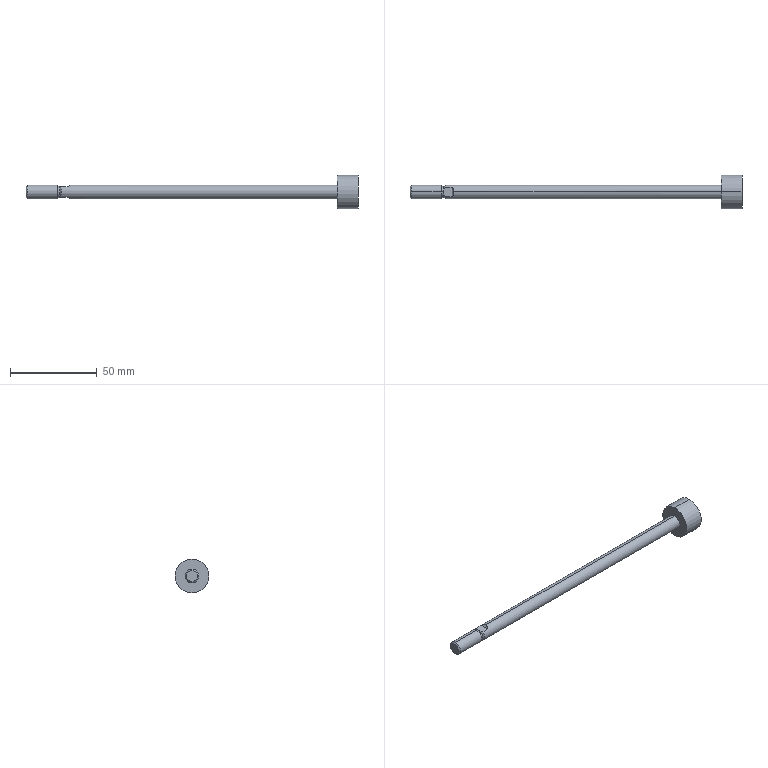Part | SolidWorks | features BaseBody 1 | 1 solid | 22 faces | box 191.2 x 19.5 x 19.5 mm | volume 12515 mm3 | plane 10 | cylinder 8 | cone 4 | commonest cylinder face diameters 8 x4 6.4 x2 19.5 x2
STEP:
#1=CARTESIAN_POINT('',(-24.5,-1.114,3.));
#2=VERTEX_POINT('',#1);
#3=CARTESIAN_POINT('',(-23.7,-2.646,3.));
#4=VERTEX_POINT('',#3);
#5=CARTESIAN_POINT('',(-24.5,-1.114,3.));
#6=CARTESIAN_POINT('',(-24.457,-1.239,3.));
#7=CARTESIAN_POINT('',(-24.38,-1.431,3.));
#8=CARTESIAN_POINT('',(-24.27,-1.665,3.));
#9=CARTESIAN_POINT('',(-24.21,-1.784,3.));
#10=CARTESIAN_POINT('',(-24.179,-1.844,3.));
#11=CARTESIAN_POINT('',(-24.165,-1.87,3.));
#12=CARTESIAN_POINT('',(-24.156,-1.887,3.));
#13=CARTESIAN_POINT('',(-24.151,-1.897,3.));
#14=CARTESIAN_POINT('',(-24.022,-2.137,3.));
#15=CARTESIAN_POINT('',(-23.873,-2.384,3.));
#16=CARTESIAN_POINT('',(-23.7,-2.646,3.));
#17=B_SPLINE_CURVE_WITH_KNOTS('',3,(#5,#6,#7,#8,#9,#10,#11,#12,#13,#14,#15,#16),.UNSPECIFIED.,.F.,.F.,(4,1,1,1,1,2,2,4),(0.,0.25,0.375,0.4375,0.4688,0.4844,0.5,1.),.UNSPECIFIED.);
#18=EDGE_CURVE('',#2,#4,#17,.T.);
#19=ORIENTED_EDGE('',*,*,#18,.T.);
#20=CARTESIAN_POINT('',(-19.7,-2.646,3.));
#21=VERTEX_POINT('',#20);
#22=CARTESIAN_POINT('',(-23.7,-2.646,3.));
#23=DIRECTION('',(1.,0.,0.));
#24=VECTOR('',#23,1000.);
#25=LINE('',#22,#24);
#26=EDGE_CURVE('',#4,#21,#25,.T.);
#27=ORIENTED_EDGE('',*,*,#26,.T.);
#28=CARTESIAN_POINT('',(-19.7,2.646,3.));
#29=VERTEX_POINT('',#28);
#30=CARTESIAN_POINT('',(-19.7,2.646,3.));
#31=DIRECTION('',(0.,-1.,0.));
#32=VECTOR('',#31,1000.);
#33=LINE('',#30,#32);
#34=EDGE_CURVE('',#29,#21,#33,.T.);
#35=ORIENTED_EDGE('',*,*,#34,.F.);
#36=CARTESIAN_POINT('',(-23.7,2.646,3.));
#37=VERTEX_POINT('',#36);
#38=CARTESIAN_POINT('',(-19.7,2.646,3.));
#39=DIRECTION('',(-1.,0.,0.));
#40=VECTOR('',#39,1000.);
#41=LINE('',#38,#40);
#42=EDGE_CURVE('',#29,#37,#41,.T.);
#43=ORIENTED_EDGE('',*,*,#42,.T.);
#44=CARTESIAN_POINT('',(-24.5,1.114,3.));
#45=VERTEX_POINT('',#44);
#46=CARTESIAN_POINT('',(-23.7,2.646,3.));
#47=CARTESIAN_POINT('',(-23.787,2.515,3.));
#48=CARTESIAN_POINT('',(-23.907,2.324,3.));
#49=CARTESIAN_POINT('',(-24.033,2.11,3.));
#50=CARTESIAN_POINT('',(-24.091,2.006,3.));
#51=CARTESIAN_POINT('',(-24.119,1.955,3.));
#52=CARTESIAN_POINT('',(-24.131,1.933,3.));
#53=CARTESIAN_POINT('',(-24.139,1.918,3.));
#54=CARTESIAN_POINT('',(-24.142,1.912,3.));
#55=CARTESIAN_POINT('',(-24.295,1.627,3.));
#56=CARTESIAN_POINT('',(-24.413,1.363,3.));
#57=CARTESIAN_POINT('',(-24.5,1.114,3.));
#58=B_SPLINE_CURVE_WITH_KNOTS('',3,(#46,#47,#48,#49,#50,#51,#52,#53,#54,#55,#56,#57),.UNSPECIFIED.,.F.,.F.,(4,1,1,1,1,2,2,4),(0.,0.25,0.375,0.4375,0.4688,0.4844,0.5,1.),.UNSPECIFIED.);
#59=EDGE_CURVE('',#37,#45,#58,.T.);
#60=ORIENTED_EDGE('',*,*,#59,.T.);
#61=CARTESIAN_POINT('',(-24.5,1.114,3.));
#62=DIRECTION('',(0.,-1.,0.));
#63=VECTOR('',#62,1000.);
#64=LINE('',#61,#63);
#65=EDGE_CURVE('',#45,#2,#64,.T.);
#66=ORIENTED_EDGE('',*,*,#65,.T.);
#67=EDGE_LOOP('',(#19,#27,#35,#43,#60,#66));
#68=FACE_OUTER_BOUND('',#67,.T.);
#69=CARTESIAN_POINT('',(-19.7,8.,3.));
#70=DIRECTION('',(0.,0.,1.));
#71=DIRECTION('',(1.,0.,0.));
#72=AXIS2_PLACEMENT_3D('',#69,#70,#71);
#73=PLANE('',#72);
#74=ADVANCED_FACE('',(#68),#73,.T.);
#75=CARTESIAN_POINT('',(-18.7,0.,4.));
#76=VERTEX_POINT('',#75);
#77=CARTESIAN_POINT('',(-19.7,-2.646,3.));
#78=CARTESIAN_POINT('',(-19.378,-2.281,3.322));
#79=CARTESIAN_POINT('',(-19.131,-1.87,3.569));
#80=CARTESIAN_POINT('',(-18.786,-0.9587,3.914));
#81=CARTESIAN_POINT('',(-18.7,-0.4873,4.));
#82=CARTESIAN_POINT('',(-18.7,0.,4.));
#83=B_SPLINE_CURVE_WITH_KNOTS('',3,(#77,#78,#79,#80,#81,#82),.UNSPECIFIED.,.F.,.F.,(4,2,4),(0.,0.5,1.),.UNSPECIFIED.);
#84=EDGE_CURVE('',#21,#76,#83,.T.);
#85=ORIENTED_EDGE('',*,*,#84,.T.);
#86=CARTESIAN_POINT('',(-18.7,0.,4.));
#87=CARTESIAN_POINT('',(-18.7,0.487,4.));
#88=CARTESIAN_POINT('',(-18.786,0.9587,3.914));
#89=CARTESIAN_POINT('',(-19.13,1.87,3.57));
#90=CARTESIAN_POINT('',(-19.378,2.28,3.322));
#91=CARTESIAN_POINT('',(-19.7,2.646,3.));
#92=B_SPLINE_CURVE_WITH_KNOTS('',3,(#86,#87,#88,#89,#90,#91),.UNSPECIFIED.,.F.,.F.,(4,2,4),(0.,0.5,1.),.UNSPECIFIED.);
#93=EDGE_CURVE('',#76,#29,#92,.T.);
#94=ORIENTED_EDGE('',*,*,#93,.T.);
#95=ORIENTED_EDGE('',*,*,#34,.T.);
#96=EDGE_LOOP('',(#85,#94,#95));
#97=FACE_OUTER_BOUND('',#96,.T.);
#98=CARTESIAN_POINT('',(-13.7,8.,9.));
#99=DIRECTION('',(-0.7071,0.,0.7071));
#100=DIRECTION('',(0.,1.,0.));
#101=AXIS2_PLACEMENT_3D('',#98,#99,#100);
#102=PLANE('',#101);
#103=ADVANCED_FACE('',(#97),#102,.T.);
#104=CARTESIAN_POINT('',(-24.5,0.,3.2));
#105=VERTEX_POINT('',#104);
#106=CARTESIAN_POINT('',(-24.5,0.,0.));
#107=DIRECTION('',(1.,0.,0.));
#108=DIRECTION('',(0.,0.348,0.9375));
#109=AXIS2_PLACEMENT_3D('',#106,#107,#108);
#110=CIRCLE('',#109,3.2);
#111=EDGE_CURVE('',#45,#105,#110,.T.);
#112=ORIENTED_EDGE('',*,*,#111,.T.);
#113=CARTESIAN_POINT('',(-24.5,0.,0.));
#114=DIRECTION('',(1.,0.,0.));
#115=DIRECTION('',(0.,0.348,0.9375));
#116=AXIS2_PLACEMENT_3D('',#113,#114,#115);
#117=CIRCLE('',#116,3.2);
#118=EDGE_CURVE('',#105,#2,#117,.T.);
#119=ORIENTED_EDGE('',*,*,#118,.T.);
#120=ORIENTED_EDGE('',*,*,#65,.F.);
#121=EDGE_LOOP('',(#112,#119,#120));
#122=FACE_OUTER_BOUND('',#121,.T.);
#123=CARTESIAN_POINT('',(-24.5,8.,3.));
#124=DIRECTION('',(1.,0.,0.));
#125=DIRECTION('',(0.,1.,0.));
#126=AXIS2_PLACEMENT_3D('',#123,#124,#125);
#127=PLANE('',#126);
#128=ADVANCED_FACE('',(#122),#127,.T.);
#129=CARTESIAN_POINT('',(-24.5,-1.114,-3.));
#130=VERTEX_POINT('',#129);
#131=CARTESIAN_POINT('',(-24.5,0.,-3.2));
#132=VERTEX_POINT('',#131);
#133=CARTESIAN_POINT('',(-24.5,0.,0.));
#134=DIRECTION('',(1.,0.,0.));
#135=DIRECTION('',(0.,-0.348,-0.9375));
#136=AXIS2_PLACEMENT_3D('',#133,#134,#135);
#137=CIRCLE('',#136,3.2);
#138=EDGE_CURVE('',#130,#132,#137,.T.);
#139=ORIENTED_EDGE('',*,*,#138,.T.);
#140=CARTESIAN_POINT('',(-24.5,1.114,-3.));
#141=VERTEX_POINT('',#140);
#142=CARTESIAN_POINT('',(-24.5,0.,0.));
#143=DIRECTION('',(1.,0.,0.));
#144=DIRECTION('',(0.,-0.348,-0.9375));
#145=AXIS2_PLACEMENT_3D('',#142,#143,#144);
#146=CIRCLE('',#145,3.2);
#147=EDGE_CURVE('',#132,#141,#146,.T.);
#148=ORIENTED_EDGE('',*,*,#147,.T.);
#149=CARTESIAN_POINT('',(-24.5,1.114,-3.));
#150=DIRECTION('',(0.,-1.,0.));
#151=VECTOR('',#150,1000.);
#152=LINE('',#149,#151);
#153=EDGE_CURVE('',#141,#130,#152,.T.);
#154=ORIENTED_EDGE('',*,*,#153,.T.);
#155=EDGE_LOOP('',(#139,#148,#154));
#156=FACE_OUTER_BOUND('',#155,.T.);
#157=CARTESIAN_POINT('',(-24.5,8.,-4.8));
#158=DIRECTION('',(1.,0.,0.));
#159=DIRECTION('',(0.,1.,0.));
#160=AXIS2_PLACEMENT_3D('',#157,#158,#159);
#161=PLANE('',#160);
#162=ADVANCED_FACE('',(#156),#161,.T.);
#163=CARTESIAN_POINT('',(-23.7,2.646,-3.));
#164=VERTEX_POINT('',#163);
#165=CARTESIAN_POINT('',(-24.5,1.114,-3.));
#166=CARTESIAN_POINT('',(-24.457,1.239,-3.));
#167=CARTESIAN_POINT('',(-24.38,1.431,-3.));
#168=CARTESIAN_POINT('',(-24.27,1.665,-3.));
#169=CARTESIAN_POINT('',(-24.21,1.784,-3.));
#170=CARTESIAN_POINT('',(-24.179,1.844,-3.));
#171=CARTESIAN_POINT('',(-24.165,1.87,-3.));
#172=CARTESIAN_POINT('',(-24.156,1.887,-3.));
#173=CARTESIAN_POINT('',(-24.151,1.897,-3.));
#174=CARTESIAN_POINT('',(-24.022,2.137,-3.));
#175=CARTESIAN_POINT('',(-23.873,2.384,-3.));
#176=CARTESIAN_POINT('',(-23.7,2.646,-3.));
#177=B_SPLINE_CURVE_WITH_KNOTS('',3,(#165,#166,#167,#168,#169,#170,#171,#172,#173,#174,#175,#176),.UNSPECIFIED.,.F.,.F.,(4,1,1,1,1,2,2,4),(0.,0.25,0.375,0.4375,0.4687,0.4844,0.5,1.),.UNSPECIFIED.);
#178=EDGE_CURVE('',#141,#164,#177,.T.);
#179=ORIENTED_EDGE('',*,*,#178,.T.);
#180=CARTESIAN_POINT('',(-19.7,2.646,-3.));
#181=VERTEX_POINT('',#180);
#182=CARTESIAN_POINT('',(-23.7,2.646,-3.));
#183=DIRECTION('',(1.,0.,0.));
#184=VECTOR('',#183,1000.);
#185=LINE('',#182,#184);
#186=EDGE_CURVE('',#164,#181,#185,.T.);
#187=ORIENTED_EDGE('',*,*,#186,.T.);
#188=CARTESIAN_POINT('',(-19.7,-2.646,-3.));
#189=VERTEX_POINT('',#188);
#190=CARTESIAN_POINT('',(-19.7,2.646,-3.));
#191=DIRECTION('',(0.,-1.,0.));
#192=VECTOR('',#191,1000.);
#193=LINE('',#190,#192);
#194=EDGE_CURVE('',#181,#189,#193,.T.);
#195=ORIENTED_EDGE('',*,*,#194,.T.);
#196=CARTESIAN_POINT('',(-23.7,-2.646,-3.));
#197=VERTEX_POINT('',#196);
#198=CARTESIAN_POINT('',(-19.7,-2.646,-3.));
#199=DIRECTION('',(-1.,0.,0.));
#200=VECTOR('',#199,1000.);
#201=LINE('',#198,#200);
#202=EDGE_CURVE('',#189,#197,#201,.T.);
#203=ORIENTED_EDGE('',*,*,#202,.T.);
#204=CARTESIAN_POINT('',(-23.7,-2.646,-3.));
#205=CARTESIAN_POINT('',(-23.787,-2.515,-3.));
#206=CARTESIAN_POINT('',(-23.907,-2.324,-3.));
#207=CARTESIAN_POINT('',(-24.033,-2.11,-3.));
#208=CARTESIAN_POINT('',(-24.091,-2.006,-3.));
#209=CARTESIAN_POINT('',(-24.119,-1.955,-3.));
#210=CARTESIAN_POINT('',(-24.131,-1.933,-3.));
#211=CARTESIAN_POINT('',(-24.139,-1.918,-3.));
#212=CARTESIAN_POINT('',(-24.142,-1.912,-3.));
#213=CARTESIAN_POINT('',(-24.295,-1.627,-3.));
#214=CARTESIAN_POINT('',(-24.413,-1.363,-3.));
#215=CARTESIAN_POINT('',(-24.5,-1.114,-3.));
#216=B_SPLINE_CURVE_WITH_KNOTS('',3,(#204,#205,#206,#207,#208,#209,#210,#211,#212,#213,#214,#215),.UNSPECIFIED.,.F.,.F.,(4,1,1,1,1,2,2,4),(0.,0.25,0.375,0.4375,0.4687,0.4844,0.5,1.),.UNSPECIFIED.);
#217=EDGE_CURVE('',#197,#130,#216,.T.);
#218=ORIENTED_EDGE('',*,*,#217,.T.);
#219=ORIENTED_EDGE('',*,*,#153,.F.);
#220=EDGE_LOOP('',(#179,#187,#195,#203,#218,#219));
#221=FACE_OUTER_BOUND('',#220,.T.);
#222=CARTESIAN_POINT('',(-24.5,8.,-3.));
#223=DIRECTION('',(0.,0.,-1.));
#224=DIRECTION('',(0.,-1.,0.));
#225=AXIS2_PLACEMENT_3D('',#222,#223,#224);
#226=PLANE('',#225);
#227=ADVANCED_FACE('',(#221),#226,.T.);
#228=CARTESIAN_POINT('',(-18.7,0.,-4.));
#229=VERTEX_POINT('',#228);
#230=CARTESIAN_POINT('',(-19.7,2.646,-3.));
#231=CARTESIAN_POINT('',(-19.378,2.281,-3.322));
#232=CARTESIAN_POINT('',(-19.131,1.87,-3.569));
#233=CARTESIAN_POINT('',(-18.786,0.9587,-3.914));
#234=CARTESIAN_POINT('',(-18.7,0.4873,-4.));
#235=CARTESIAN_POINT('',(-18.7,0.,-4.));
#236=B_SPLINE_CURVE_WITH_KNOTS('',3,(#230,#231,#232,#233,#234,#235),.UNSPECIFIED.,.F.,.F.,(4,2,4),(0.,0.5,1.),.UNSPECIFIED.);
#237=EDGE_CURVE('',#181,#229,#236,.T.);
#238=ORIENTED_EDGE('',*,*,#237,.T.);
#239=CARTESIAN_POINT('',(-18.7,0.,-4.));
#240=CARTESIAN_POINT('',(-18.7,-0.487,-4.));
#241=CARTESIAN_POINT('',(-18.786,-0.9587,-3.914));
#242=CARTESIAN_POINT('',(-19.13,-1.87,-3.57));
#243=CARTESIAN_POINT('',(-19.378,-2.28,-3.322));
#244=CARTESIAN_POINT('',(-19.7,-2.646,-3.));
#245=B_SPLINE_CURVE_WITH_KNOTS('',3,(#239,#240,#241,#242,#243,#244),.UNSPECIFIED.,.F.,.F.,(4,2,4),(0.,0.5,1.),.UNSPECIFIED.);
#246=EDGE_CURVE('',#229,#189,#245,.T.);
#247=ORIENTED_EDGE('',*,*,#246,.T.);
#248=ORIENTED_EDGE('',*,*,#194,.F.);
#249=EDGE_LOOP('',(#238,#247,#248));
#250=FACE_OUTER_BOUND('',#249,.T.);
#251=CARTESIAN_POINT('',(-19.7,8.,-3.));
#252=DIRECTION('',(-0.7071,0.,-0.7071));
#253=DIRECTION('',(-0.7071,0.,0.7071));
#254=AXIS2_PLACEMENT_3D('',#251,#252,#253);
#255=PLANE('',#254);
#256=ADVANCED_FACE('',(#250),#255,.T.);
#257=CARTESIAN_POINT('',(147.2,0.,-9.75));
#258=VERTEX_POINT('',#257);
#259=CARTESIAN_POINT('',(147.2,0.,9.75));
#260=VERTEX_POINT('',#259);
#261=CARTESIAN_POINT('',(147.2,0.,0.));
#262=DIRECTION('',(1.,0.,0.));
#263=DIRECTION('',(0.,0.,-1.));
#264=AXIS2_PLACEMENT_3D('',#261,#262,#263);
#265=CIRCLE('',#264,9.75);
#266=EDGE_CURVE('',#258,#260,#265,.T.);
#267=ORIENTED_EDGE('',*,*,#266,.T.);
#268=CARTESIAN_POINT('',(147.2,0.,0.));
#269=DIRECTION('',(1.,0.,0.));
#270=DIRECTION('',(0.,0.,-1.));
#271=AXIS2_PLACEMENT_3D('',#268,#269,#270);
#272=CIRCLE('',#271,9.75);
#273=EDGE_CURVE('',#260,#258,#272,.T.);
#274=ORIENTED_EDGE('',*,*,#273,.T.);
#275=EDGE_LOOP('',(#267,#274));
#276=FACE_OUTER_BOUND('',#275,.T.);
#277=CARTESIAN_POINT('',(147.2,9.75,0.));
#278=DIRECTION('',(-1.,0.,0.));
#279=DIRECTION('',(0.,0.,1.));
#280=AXIS2_PLACEMENT_3D('',#277,#278,#279);
#281=PLANE('',#280);
#282=ADVANCED_FACE('',(#276),#281,.F.);
#283=CARTESIAN_POINT('',(135.2,0.,9.75));
#284=VERTEX_POINT('',#283);
#285=CARTESIAN_POINT('',(147.2,0.,9.75));
#286=DIRECTION('',(1.,0.,0.));
#287=VECTOR('',#286,1000.);
#288=LINE('',#285,#287);
#289=EDGE_CURVE('',#284,#260,#288,.T.);
#290=ORIENTED_EDGE('',*,*,#289,.F.);
#291=CARTESIAN_POINT('',(135.2,0.,-9.75));
#292=VERTEX_POINT('',#291);
#293=CARTESIAN_POINT('',(135.2,0.,0.));
#294=DIRECTION('',(1.,0.,0.));
#295=DIRECTION('',(0.,0.,-1.));
#296=AXIS2_PLACEMENT_3D('',#293,#294,#295);
#297=CIRCLE('',#296,9.75);
#298=EDGE_CURVE('',#284,#292,#297,.T.);
#299=ORIENTED_EDGE('',*,*,#298,.T.);
#300=CARTESIAN_POINT('',(147.2,0.,-9.75));
#301=DIRECTION('',(1.,0.,0.));
#302=VECTOR('',#301,1000.);
#303=LINE('',#300,#302);
#304=EDGE_CURVE('',#292,#258,#303,.T.);
#305=ORIENTED_EDGE('',*,*,#304,.T.);
#306=ORIENTED_EDGE('',*,*,#273,.F.);
#307=EDGE_LOOP('',(#290,#299,#305,#306));
#308=FACE_OUTER_BOUND('',#307,.T.);
#309=CARTESIAN_POINT('',(147.2,0.,0.));
#310=DIRECTION('',(1.,0.,0.));
#311=DIRECTION('',(0.,0.,-1.));
#312=AXIS2_PLACEMENT_3D('',#309,#310,#311);
#313=CYLINDRICAL_SURFACE('',#312,9.75);
#314=ADVANCED_FACE('',(#308),#313,.T.);
#315=CARTESIAN_POINT('',(135.2,0.,-4.));
#316=VERTEX_POINT('',#315);
#317=CARTESIAN_POINT('',(135.2,0.,4.));
#318=VERTEX_POINT('',#317);
#319=CARTESIAN_POINT('',(135.2,0.,0.));
#320=DIRECTION('',(1.,0.,0.));
#321=DIRECTION('',(0.,0.,-1.));
#322=AXIS2_PLACEMENT_3D('',#319,#320,#321);
#323=CIRCLE('',#322,4.);
#324=EDGE_CURVE('',#316,#318,#323,.T.);
#325=ORIENTED_EDGE('',*,*,#324,.T.);
#326=CARTESIAN_POINT('',(135.2,0.,0.));
#327=DIRECTION('',(1.,0.,0.));
#328=DIRECTION('',(0.,0.,-1.));
#329=AXIS2_PLACEMENT_3D('',#326,#327,#328);
#330=CIRCLE('',#329,4.);
#331=EDGE_CURVE('',#318,#316,#330,.T.);
#332=ORIENTED_EDGE('',*,*,#331,.T.);
#333=EDGE_LOOP('',(#325,#332));
#334=FACE_BOUND('',#333,.T.);
#335=CARTESIAN_POINT('',(135.2,0.,0.));
#336=DIRECTION('',(1.,0.,0.));
#337=DIRECTION('',(0.,0.,-1.));
#338=AXIS2_PLACEMENT_3D('',#335,#336,#337);
#339=CIRCLE('',#338,9.75);
#340=EDGE_CURVE('',#292,#284,#339,.T.);
#341=ORIENTED_EDGE('',*,*,#340,.F.);
#342=ORIENTED_EDGE('',*,*,#298,.F.);
#343=EDGE_LOOP('',(#341,#342));
#344=FACE_OUTER_BOUND('',#343,.T.);
#345=CARTESIAN_POINT('',(135.2,4.,0.));
#346=DIRECTION('',(1.,0.,0.));
#347=DIRECTION('',(0.,1.,0.));
#348=AXIS2_PLACEMENT_3D('',#345,#346,#347);
#349=PLANE('',#348);
#350=ADVANCED_FACE('',(#334,#344),#349,.F.);
#351=CARTESIAN_POINT('',(-26.,0.,3.2));
#352=VERTEX_POINT('',#351);
#353=CARTESIAN_POINT('',(147.2,0.,3.2));
#354=DIRECTION('',(1.,0.,0.));
#355=VECTOR('',#354,1000.);
#356=LINE('',#353,#355);
#357=EDGE_CURVE('',#352,#105,#356,.T.);
#358=ORIENTED_EDGE('',*,*,#357,.F.);
#359=CARTESIAN_POINT('',(-26.,0.,-3.2));
#360=VERTEX_POINT('',#359);
#361=CARTESIAN_POINT('',(-26.,0.,0.));
#362=DIRECTION('',(1.,0.,0.));
#363=DIRECTION('',(0.,0.,-1.));
#364=AXIS2_PLACEMENT_3D('',#361,#362,#363);
#365=CIRCLE('',#364,3.2);
#366=EDGE_CURVE('',#352,#360,#365,.T.);
#367=ORIENTED_EDGE('',*,*,#366,.T.);
#368=CARTESIAN_POINT('',(147.2,0.,-3.2));
#369=DIRECTION('',(1.,0.,0.));
#370=VECTOR('',#369,1000.);
#371=LINE('',#368,#370);
#372=EDGE_CURVE('',#360,#132,#371,.T.);
#373=ORIENTED_EDGE('',*,*,#372,.T.);
#374=ORIENTED_EDGE('',*,*,#138,.F.);
#375=CARTESIAN_POINT('',(-24.5,0.,0.));
#376=DIRECTION('',(1.,0.,0.));
#377=DIRECTION('',(0.,-0.348,0.9375));
#378=AXIS2_PLACEMENT_3D('',#375,#376,#377);
#379=CIRCLE('',#378,3.2);
#380=EDGE_CURVE('',#2,#130,#379,.T.);
#381=ORIENTED_EDGE('',*,*,#380,.F.);
#382=ORIENTED_EDGE('',*,*,#118,.F.);
#383=EDGE_LOOP('',(#358,#367,#373,#374,#381,#382));
#384=FACE_OUTER_BOUND('',#383,.T.);
#385=CARTESIAN_POINT('',(147.2,0.,0.));
#386=DIRECTION('',(1.,0.,0.));
#387=DIRECTION('',(0.,0.,-1.));
#388=AXIS2_PLACEMENT_3D('',#385,#386,#387);
#389=CYLINDRICAL_SURFACE('',#388,3.2);
#390=ADVANCED_FACE('',(#384),#389,.T.);
#391=CARTESIAN_POINT('',(-26.,0.,0.));
#392=DIRECTION('',(1.,0.,0.));
#393=DIRECTION('',(0.,0.,-1.));
#394=AXIS2_PLACEMENT_3D('',#391,#392,#393);
#395=CIRCLE('',#394,3.2);
#396=EDGE_CURVE('',#360,#352,#395,.T.);
#397=ORIENTED_EDGE('',*,*,#396,.F.);
#398=ORIENTED_EDGE('',*,*,#366,.F.);
#399=EDGE_LOOP('',(#397,#398));
#400=FACE_BOUND('',#399,.T.);
#401=CARTESIAN_POINT('',(-26.,0.,-4.));
#402=VERTEX_POINT('',#401);
#403=CARTESIAN_POINT('',(-26.,0.,4.));
#404=VERTEX_POINT('',#403);
#405=CARTESIAN_POINT('',(-26.,0.,0.));
#406=DIRECTION('',(1.,0.,0.));
#407=DIRECTION('',(0.,0.,-1.));
#408=AXIS2_PLACEMENT_3D('',#405,#406,#407);
#409=CIRCLE('',#408,4.);
#410=EDGE_CURVE('',#402,#404,#409,.T.);
#411=ORIENTED_EDGE('',*,*,#410,.T.);
#412=CARTESIAN_POINT('',(-26.,0.,0.));
#413=DIRECTION('',(1.,0.,0.));
#414=DIRECTION('',(0.,0.,-1.));
#415=AXIS2_PLACEMENT_3D('',#412,#413,#414);
#416=CIRCLE('',#415,4.);
#417=EDGE_CURVE('',#404,#402,#416,.T.);
#418=ORIENTED_EDGE('',*,*,#417,.T.);
#419=EDGE_LOOP('',(#411,#418));
#420=FACE_OUTER_BOUND('',#419,.T.);
#421=CARTESIAN_POINT('',(-26.,4.,0.));
#422=DIRECTION('',(-1.,0.,0.));
#423=DIRECTION('',(0.,0.,1.));
#424=AXIS2_PLACEMENT_3D('',#421,#422,#423);
#425=PLANE('',#424);
#426=ADVANCED_FACE('',(#400,#420),#425,.F.);
#427=CARTESIAN_POINT('',(-43.233,0.,4.));
#428=VERTEX_POINT('',#427);
#429=CARTESIAN_POINT('',(147.2,0.,4.));
#430=DIRECTION('',(1.,0.,0.));
#431=VECTOR('',#430,1000.);
#432=LINE('',#429,#431);
#433=EDGE_CURVE('',#428,#404,#432,.T.);
#434=ORIENTED_EDGE('',*,*,#433,.F.);
#435=CARTESIAN_POINT('',(-43.233,0.,-4.));
#436=VERTEX_POINT('',#435);
#437=CARTESIAN_POINT('',(-43.233,0.,0.));
#438=DIRECTION('',(1.,0.,0.));
#439=DIRECTION('',(0.,0.,-1.));
#440=AXIS2_PLACEMENT_3D('',#437,#438,#439);
#441=CIRCLE('',#440,4.);
#442=EDGE_CURVE('',#428,#436,#441,.T.);
#443=ORIENTED_EDGE('',*,*,#442,.T.);
#444=CARTESIAN_POINT('',(147.2,0.,-4.));
#445=DIRECTION('',(1.,0.,0.));
#446=VECTOR('',#445,1000.);
#447=LINE('',#444,#446);
#448=EDGE_CURVE('',#436,#402,#447,.T.);
#449=ORIENTED_EDGE('',*,*,#448,.T.);
#450=ORIENTED_EDGE('',*,*,#417,.F.);
#451=EDGE_LOOP('',(#434,#443,#449,#450));
#452=FACE_OUTER_BOUND('',#451,.T.);
#453=CARTESIAN_POINT('',(147.2,0.,0.));
#454=DIRECTION('',(1.,0.,0.));
#455=DIRECTION('',(0.,0.,-1.));
#456=AXIS2_PLACEMENT_3D('',#453,#454,#455);
#457=CYLINDRICAL_SURFACE('',#456,4.);
#458=ADVANCED_FACE('',(#452),#457,.T.);
#459=CARTESIAN_POINT('',(-44.,0.,3.233));
#460=VERTEX_POINT('',#459);
#461=CARTESIAN_POINT('',(-44.,0.,3.233));
#462=DIRECTION('',(0.7071,0.,0.7071));
#463=VECTOR('',#462,1000.);
#464=LINE('',#461,#463);
#465=EDGE_CURVE('',#460,#428,#464,.T.);
#466=ORIENTED_EDGE('',*,*,#465,.F.);
#467=CARTESIAN_POINT('',(-44.,0.,-3.233));
#468=VERTEX_POINT('',#467);
#469=CARTESIAN_POINT('',(-44.,0.,0.));
#470=DIRECTION('',(1.,0.,0.));
#471=DIRECTION('',(0.,0.,-1.));
#472=AXIS2_PLACEMENT_3D('',#469,#470,#471);
#473=CIRCLE('',#472,3.233);
#474=EDGE_CURVE('',#460,#468,#473,.T.);
#475=ORIENTED_EDGE('',*,*,#474,.T.);
#476=CARTESIAN_POINT('',(-44.,0.,-3.233));
#477=DIRECTION('',(0.7071,0.,-0.7071));
#478=VECTOR('',#477,1000.);
#479=LINE('',#476,#478);
#480=EDGE_CURVE('',#468,#436,#479,.T.);
#481=ORIENTED_EDGE('',*,*,#480,.T.);
#482=ORIENTED_EDGE('',*,*,#442,.F.);
#483=EDGE_LOOP('',(#466,#475,#481,#482));
#484=FACE_OUTER_BOUND('',#483,.T.);
#485=CARTESIAN_POINT('',(-44.,0.,0.));
#486=DIRECTION('',(1.,0.,0.));
#487=DIRECTION('',(0.,0.,-1.));
#488=AXIS2_PLACEMENT_3D('',#485,#486,#487);
#489=CONICAL_SURFACE('',#488,3.233,0.7854);
#490=ADVANCED_FACE('',(#484),#489,.T.);
#491=CARTESIAN_POINT('',(-44.,0.,0.));
#492=DIRECTION('',(1.,0.,0.));
#493=DIRECTION('',(0.,0.,-1.));
#494=AXIS2_PLACEMENT_3D('',#491,#492,#493);
#495=CIRCLE('',#494,3.233);
#496=EDGE_CURVE('',#468,#460,#495,.T.);
#497=ORIENTED_EDGE('',*,*,#496,.F.);
#498=ORIENTED_EDGE('',*,*,#474,.F.);
#499=EDGE_LOOP('',(#497,#498));
#500=FACE_OUTER_BOUND('',#499,.T.);
#501=CARTESIAN_POINT('',(-44.,0.,0.));
#502=DIRECTION('',(1.,0.,0.));
#503=DIRECTION('',(0.,1.,0.));
#504=AXIS2_PLACEMENT_3D('',#501,#502,#503);
#505=PLANE('',#504);
#506=ADVANCED_FACE('',(#500),#505,.F.);
#507=CARTESIAN_POINT('',(147.2,0.,4.));
#508=DIRECTION('',(1.,0.,0.));
#509=VECTOR('',#508,1000.);
#510=LINE('',#507,#509);
#511=EDGE_CURVE('',#76,#318,#510,.T.);
#512=ORIENTED_EDGE('',*,*,#511,.F.);
#513=ORIENTED_EDGE('',*,*,#84,.F.);
#514=ORIENTED_EDGE('',*,*,#26,.F.);
#515=CARTESIAN_POINT('',(-23.7,0.,0.));
#516=DIRECTION('',(1.,0.,0.));
#517=DIRECTION('',(0.,-0.6614,0.75));
#518=AXIS2_PLACEMENT_3D('',#515,#516,#517);
#519=CIRCLE('',#518,4.);
#520=EDGE_CURVE('',#4,#197,#519,.T.);
#521=ORIENTED_EDGE('',*,*,#520,.T.);
#522=ORIENTED_EDGE('',*,*,#202,.F.);
#523=ORIENTED_EDGE('',*,*,#246,.F.);
#524=CARTESIAN_POINT('',(147.2,0.,-4.));
#525=DIRECTION('',(1.,0.,0.));
#526=VECTOR('',#525,1000.);
#527=LINE('',#524,#526);
#528=EDGE_CURVE('',#229,#316,#527,.T.);
#529=ORIENTED_EDGE('',*,*,#528,.T.);
#530=ORIENTED_EDGE('',*,*,#331,.F.);
#531=EDGE_LOOP('',(#512,#513,#514,#521,#522,#523,#529,#530));
#532=FACE_OUTER_BOUND('',#531,.T.);
#533=CARTESIAN_POINT('',(147.2,0.,0.));
#534=DIRECTION('',(1.,0.,0.));
#535=DIRECTION('',(0.,0.,-1.));
#536=AXIS2_PLACEMENT_3D('',#533,#534,#535);
#537=CYLINDRICAL_SURFACE('',#536,4.);
#538=ADVANCED_FACE('',(#532),#537,.T.);
#539=ORIENTED_EDGE('',*,*,#18,.F.);
#540=ORIENTED_EDGE('',*,*,#380,.T.);
#541=ORIENTED_EDGE('',*,*,#217,.F.);
#542=ORIENTED_EDGE('',*,*,#520,.F.);
#543=EDGE_LOOP('',(#539,#540,#541,#542));
#544=FACE_OUTER_BOUND('',#543,.T.);
#545=CARTESIAN_POINT('',(-24.5,0.,0.));
#546=DIRECTION('',(1.,0.,0.));
#547=DIRECTION('',(0.,0.,-1.));
#548=AXIS2_PLACEMENT_3D('',#545,#546,#547);
#549=CONICAL_SURFACE('',#548,3.2,0.7854);
#550=ADVANCED_FACE('',(#544),#549,.T.);
#551=ORIENTED_EDGE('',*,*,#59,.F.);
#552=CARTESIAN_POINT('',(-23.7,0.,0.));
#553=DIRECTION('',(1.,0.,0.));
#554=DIRECTION('',(0.,0.6614,-0.75));
#555=AXIS2_PLACEMENT_3D('',#552,#553,#554);
#556=CIRCLE('',#555,4.);
#557=EDGE_CURVE('',#164,#37,#556,.T.);
#558=ORIENTED_EDGE('',*,*,#557,.F.);
#559=ORIENTED_EDGE('',*,*,#178,.F.);
#560=CARTESIAN_POINT('',(-24.5,0.,0.));
#561=DIRECTION('',(1.,0.,0.));
#562=DIRECTION('',(0.,0.348,-0.9375));
#563=AXIS2_PLACEMENT_3D('',#560,#561,#562);
#564=CIRCLE('',#563,3.2);
#565=EDGE_CURVE('',#141,#45,#564,.T.);
#566=ORIENTED_EDGE('',*,*,#565,.T.);
#567=EDGE_LOOP('',(#551,#558,#559,#566));
#568=FACE_OUTER_BOUND('',#567,.T.);
#569=CARTESIAN_POINT('',(-24.5,0.,0.));
#570=DIRECTION('',(1.,0.,0.));
#571=DIRECTION('',(0.,0.,-1.));
#572=AXIS2_PLACEMENT_3D('',#569,#570,#571);
#573=CONICAL_SURFACE('',#572,3.2,0.7854);
#574=ADVANCED_FACE('',(#568),#573,.T.);
#575=ORIENTED_EDGE('',*,*,#93,.F.);
#576=ORIENTED_EDGE('',*,*,#511,.T.);
#577=ORIENTED_EDGE('',*,*,#324,.F.);
#578=ORIENTED_EDGE('',*,*,#528,.F.);
#579=ORIENTED_EDGE('',*,*,#237,.F.);
#580=ORIENTED_EDGE('',*,*,#186,.F.);
#581=ORIENTED_EDGE('',*,*,#557,.T.);
#582=ORIENTED_EDGE('',*,*,#42,.F.);
#583=EDGE_LOOP('',(#575,#576,#577,#578,#579,#580,#581,#582));
#584=FACE_OUTER_BOUND('',#583,.T.);
#585=CARTESIAN_POINT('',(147.2,0.,0.));
#586=DIRECTION('',(1.,0.,0.));
#587=DIRECTION('',(0.,0.,-1.));
#588=AXIS2_PLACEMENT_3D('',#585,#586,#587);
#589=CYLINDRICAL_SURFACE('',#588,4.);
#590=ADVANCED_FACE('',(#584),#589,.T.);
#591=ORIENTED_EDGE('',*,*,#496,.T.);
#592=ORIENTED_EDGE('',*,*,#465,.T.);
#593=CARTESIAN_POINT('',(-43.233,0.,0.));
#594=DIRECTION('',(1.,0.,0.));
#595=DIRECTION('',(0.,0.,-1.));
#596=AXIS2_PLACEMENT_3D('',#593,#594,#595);
#597=CIRCLE('',#596,4.);
#598=EDGE_CURVE('',#436,#428,#597,.T.);
#599=ORIENTED_EDGE('',*,*,#598,.F.);
#600=ORIENTED_EDGE('',*,*,#480,.F.);
#601=EDGE_LOOP('',(#591,#592,#599,#600));
#602=FACE_OUTER_BOUND('',#601,.T.);
#603=CARTESIAN_POINT('',(-44.,0.,0.));
#604=DIRECTION('',(1.,0.,0.));
#605=DIRECTION('',(0.,0.,-1.));
#606=AXIS2_PLACEMENT_3D('',#603,#604,#605);
#607=CONICAL_SURFACE('',#606,3.233,0.7854);
#608=ADVANCED_FACE('',(#602),#607,.T.);
#609=ORIENTED_EDGE('',*,*,#598,.T.);
#610=ORIENTED_EDGE('',*,*,#433,.T.);
#611=ORIENTED_EDGE('',*,*,#410,.F.);
#612=ORIENTED_EDGE('',*,*,#448,.F.);
#613=EDGE_LOOP('',(#609,#610,#611,#612));
#614=FACE_OUTER_BOUND('',#613,.T.);
#615=CARTESIAN_POINT('',(147.2,0.,0.));
#616=DIRECTION('',(1.,0.,0.));
#617=DIRECTION('',(0.,0.,-1.));
#618=AXIS2_PLACEMENT_3D('',#615,#616,#617);
#619=CYLINDRICAL_SURFACE('',#618,4.);
#620=ADVANCED_FACE('',(#614),#619,.T.);
#621=ORIENTED_EDGE('',*,*,#396,.T.);
#622=ORIENTED_EDGE('',*,*,#357,.T.);
#623=ORIENTED_EDGE('',*,*,#111,.F.);
#624=ORIENTED_EDGE('',*,*,#565,.F.);
#625=ORIENTED_EDGE('',*,*,#147,.F.);
#626=ORIENTED_EDGE('',*,*,#372,.F.);
#627=EDGE_LOOP('',(#621,#622,#623,#624,#625,#626));
#628=FACE_OUTER_BOUND('',#627,.T.);
#629=CARTESIAN_POINT('',(147.2,0.,0.));
#630=DIRECTION('',(1.,0.,0.));
#631=DIRECTION('',(0.,0.,-1.));
#632=AXIS2_PLACEMENT_3D('',#629,#630,#631);
#633=CYLINDRICAL_SURFACE('',#632,3.2);
#634=ADVANCED_FACE('',(#628),#633,.T.);
#635=ORIENTED_EDGE('',*,*,#340,.T.);
#636=ORIENTED_EDGE('',*,*,#289,.T.);
#637=ORIENTED_EDGE('',*,*,#266,.F.);
#638=ORIENTED_EDGE('',*,*,#304,.F.);
#639=EDGE_LOOP('',(#635,#636,#637,#638));
#640=FACE_OUTER_BOUND('',#639,.T.);
#641=CARTESIAN_POINT('',(147.2,0.,0.));
#642=DIRECTION('',(1.,0.,0.));
#643=DIRECTION('',(0.,0.,-1.));
#644=AXIS2_PLACEMENT_3D('',#641,#642,#643);
#645=CYLINDRICAL_SURFACE('',#644,9.75);
#646=ADVANCED_FACE('',(#640),#645,.T.);
#647=CLOSED_SHELL('',(#74,#103,#128,#162,#227,#256,#282,#314,#350,#390,#426,#458,#490,#506,#538,#550,#574,#590,#608,#620,#634,#646));
#648=MANIFOLD_SOLID_BREP('',#647);
#649=CARTESIAN_POINT('',(0.,0.,0.));
#650=DIRECTION('',(0.,0.,1.));
#651=DIRECTION('',(1.,0.,0.));
#652=AXIS2_PLACEMENT_3D('',#649,#650,#651);
#653=(LENGTH_UNIT()NAMED_UNIT(*)SI_UNIT(.MILLI.,.METRE.));
#654=UNCERTAINTY_MEASURE_WITH_UNIT(LENGTH_MEASURE(0.00001),#653,'','');
#655=(NAMED_UNIT(*)PLANE_ANGLE_UNIT()SI_UNIT($,.RADIAN.));
#656=(NAMED_UNIT(*)SI_UNIT($,.STERADIAN.)SOLID_ANGLE_UNIT());
#657=(GEOMETRIC_REPRESENTATION_CONTEXT(3)GLOBAL_UNCERTAINTY_ASSIGNED_CONTEXT((#654))GLOBAL_UNIT_ASSIGNED_CONTEXT((#653,#655,#656))REPRESENTATION_CONTEXT('',''));
#658=ADVANCED_BREP_SHAPE_REPRESENTATION('',(#648,#652),#657);